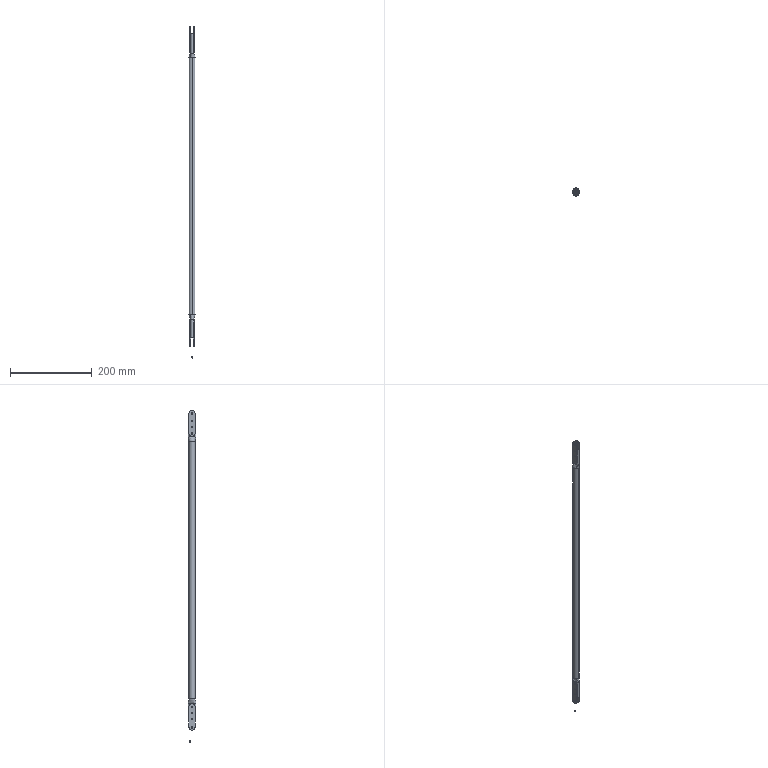Part | SolidWorks | features BaseBody 10 | 10 solids | 106 faces | box 15.875 x 19.559 x 814.088 mm | volume 36752 mm3 | cylinder 62 | plane 32 | spline 12 | commonest cylinder face diameters 3.175 x18 3.2 x16 15 x12 4.826 x8 6.858 x4 14.097 x2